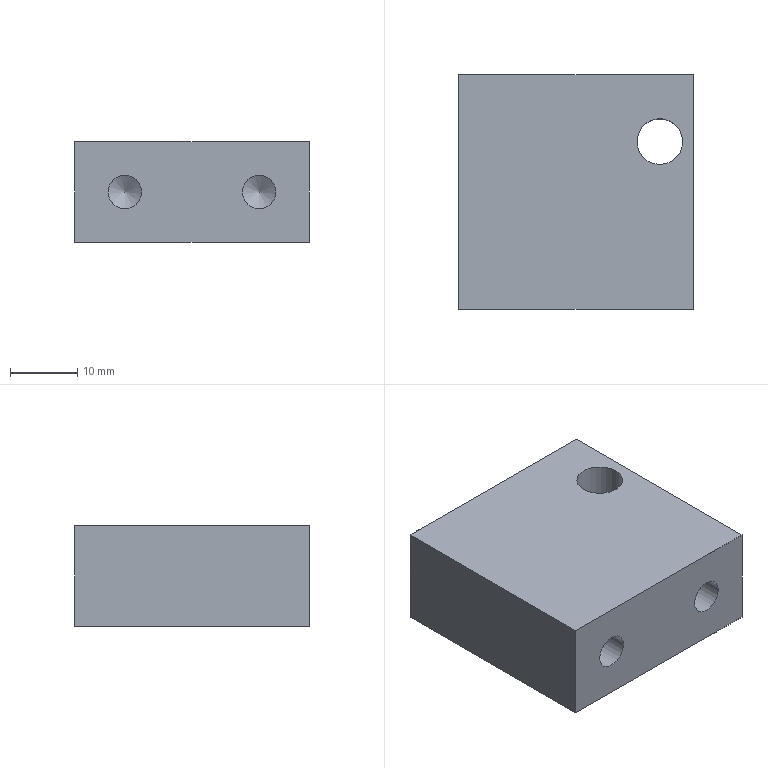Part | NX | features 5003_216_Bracket 2 | 1 solid | 11 faces | box 35 x 35 x 15 mm | volume 17222 mm3 | plane 6 | cylinder 3 | cone 2 | commonest cylinder face diameters 5 x2 6.8 x1
STEP:
#1=CARTESIAN_POINT('',(-185.615,28.9,-84.5));
#2=VERTEX_POINT('',#1);
#3=CARTESIAN_POINT('',(-185.615,-6.1,-84.5));
#4=VERTEX_POINT('',#3);
#5=CARTESIAN_POINT('',(-185.615,-6.1,-84.5));
#6=DIRECTION('',(0.,-1.,0.));
#7=VECTOR('',#6,1000.);
#8=LINE('',#5,#7);
#9=EDGE_CURVE('',#2,#4,#8,.T.);
#10=ORIENTED_EDGE('',*,*,#9,.T.);
#11=CARTESIAN_POINT('',(-185.615,-6.1,-69.5));
#12=VERTEX_POINT('',#11);
#13=CARTESIAN_POINT('',(-185.615,-6.1,-69.5));
#14=DIRECTION('',(0.,0.,-1.));
#15=VECTOR('',#14,1000.);
#16=LINE('',#13,#15);
#17=EDGE_CURVE('',#12,#4,#16,.T.);
#18=ORIENTED_EDGE('',*,*,#17,.F.);
#19=CARTESIAN_POINT('',(-185.615,28.9,-69.5));
#20=VERTEX_POINT('',#19);
#21=CARTESIAN_POINT('',(-185.615,-6.1,-69.5));
#22=DIRECTION('',(0.,-1.,0.));
#23=VECTOR('',#22,1000.);
#24=LINE('',#21,#23);
#25=EDGE_CURVE('',#20,#12,#24,.T.);
#26=ORIENTED_EDGE('',*,*,#25,.F.);
#27=CARTESIAN_POINT('',(-185.615,28.9,-69.5));
#28=DIRECTION('',(0.,0.,-1.));
#29=VECTOR('',#28,1000.);
#30=LINE('',#27,#29);
#31=EDGE_CURVE('',#20,#2,#30,.T.);
#32=ORIENTED_EDGE('',*,*,#31,.T.);
#33=EDGE_LOOP('',(#10,#18,#26,#32));
#34=FACE_BOUND('',#33,.T.);
#35=CARTESIAN_POINT('',(-185.615,-6.1,-69.5));
#36=DIRECTION('',(1.,0.,0.));
#37=DIRECTION('',(0.,0.,-1.));
#38=AXIS2_PLACEMENT_3D('',#35,#36,#37);
#39=PLANE('',#38);
#40=ADVANCED_FACE('',(#34),#39,.F.);
#41=CARTESIAN_POINT('',(-178.115,-6.1,-79.5));
#42=VERTEX_POINT('',#41);
#43=CARTESIAN_POINT('',(-178.115,-6.1,-77.));
#44=DIRECTION('',(0.,-1.,0.));
#45=DIRECTION('',(0.,0.,-1.));
#46=AXIS2_PLACEMENT_3D('',#43,#44,#45);
#47=CIRCLE('',#46,2.5);
#48=EDGE_CURVE('',#42,#42,#47,.T.);
#49=ORIENTED_EDGE('',*,*,#48,.F.);
#50=EDGE_LOOP('',(#49));
#51=FACE_BOUND('',#50,.T.);
#52=CARTESIAN_POINT('',(-158.115,-6.1,-79.5));
#53=VERTEX_POINT('',#52);
#54=CARTESIAN_POINT('',(-158.115,-6.1,-77.));
#55=DIRECTION('',(0.,-1.,0.));
#56=DIRECTION('',(0.,0.,-1.));
#57=AXIS2_PLACEMENT_3D('',#54,#55,#56);
#58=CIRCLE('',#57,2.5);
#59=EDGE_CURVE('',#53,#53,#58,.T.);
#60=ORIENTED_EDGE('',*,*,#59,.F.);
#61=EDGE_LOOP('',(#60));
#62=FACE_BOUND('',#61,.T.);
#63=CARTESIAN_POINT('',(-150.615,-6.1,-84.5));
#64=VERTEX_POINT('',#63);
#65=CARTESIAN_POINT('',(-150.615,-6.1,-84.5));
#66=DIRECTION('',(1.,0.,0.));
#67=VECTOR('',#66,1000.);
#68=LINE('',#65,#67);
#69=EDGE_CURVE('',#4,#64,#68,.T.);
#70=ORIENTED_EDGE('',*,*,#69,.T.);
#71=CARTESIAN_POINT('',(-150.615,-6.1,-69.5));
#72=VERTEX_POINT('',#71);
#73=CARTESIAN_POINT('',(-150.615,-6.1,-69.5));
#74=DIRECTION('',(0.,0.,-1.));
#75=VECTOR('',#74,1000.);
#76=LINE('',#73,#75);
#77=EDGE_CURVE('',#72,#64,#76,.T.);
#78=ORIENTED_EDGE('',*,*,#77,.F.);
#79=CARTESIAN_POINT('',(-150.615,-6.1,-69.5));
#80=DIRECTION('',(1.,0.,0.));
#81=VECTOR('',#80,1000.);
#82=LINE('',#79,#81);
#83=EDGE_CURVE('',#12,#72,#82,.T.);
#84=ORIENTED_EDGE('',*,*,#83,.F.);
#85=ORIENTED_EDGE('',*,*,#17,.T.);
#86=EDGE_LOOP('',(#70,#78,#84,#85));
#87=FACE_BOUND('',#86,.T.);
#88=CARTESIAN_POINT('',(-150.615,-6.1,-69.5));
#89=DIRECTION('',(0.,1.,0.));
#90=DIRECTION('',(-1.,0.,0.));
#91=AXIS2_PLACEMENT_3D('',#88,#89,#90);
#92=PLANE('',#91);
#93=ADVANCED_FACE('',(#51,#62,#87),#92,.F.);
#94=CARTESIAN_POINT('',(-150.615,28.9,-84.5));
#95=VERTEX_POINT('',#94);
#96=CARTESIAN_POINT('',(-150.615,-6.1,-84.5));
#97=DIRECTION('',(0.,1.,0.));
#98=VECTOR('',#97,1000.);
#99=LINE('',#96,#98);
#100=EDGE_CURVE('',#64,#95,#99,.T.);
#101=ORIENTED_EDGE('',*,*,#100,.T.);
#102=CARTESIAN_POINT('',(-150.615,28.9,-69.5));
#103=VERTEX_POINT('',#102);
#104=CARTESIAN_POINT('',(-150.615,28.9,-69.5));
#105=DIRECTION('',(0.,0.,-1.));
#106=VECTOR('',#105,1000.);
#107=LINE('',#104,#106);
#108=EDGE_CURVE('',#103,#95,#107,.T.);
#109=ORIENTED_EDGE('',*,*,#108,.F.);
#110=CARTESIAN_POINT('',(-150.615,-6.1,-69.5));
#111=DIRECTION('',(0.,1.,0.));
#112=VECTOR('',#111,1000.);
#113=LINE('',#110,#112);
#114=EDGE_CURVE('',#72,#103,#113,.T.);
#115=ORIENTED_EDGE('',*,*,#114,.F.);
#116=ORIENTED_EDGE('',*,*,#77,.T.);
#117=EDGE_LOOP('',(#101,#109,#115,#116));
#118=FACE_BOUND('',#117,.T.);
#119=CARTESIAN_POINT('',(-150.615,-6.1,-69.5));
#120=DIRECTION('',(-1.,0.,0.));
#121=DIRECTION('',(0.,0.,1.));
#122=AXIS2_PLACEMENT_3D('',#119,#120,#121);
#123=PLANE('',#122);
#124=ADVANCED_FACE('',(#118),#123,.F.);
#125=CARTESIAN_POINT('',(-150.615,28.9,-84.5));
#126=DIRECTION('',(-1.,0.,0.));
#127=VECTOR('',#126,1000.);
#128=LINE('',#125,#127);
#129=EDGE_CURVE('',#95,#2,#128,.T.);
#130=ORIENTED_EDGE('',*,*,#129,.T.);
#131=ORIENTED_EDGE('',*,*,#31,.F.);
#132=CARTESIAN_POINT('',(-150.615,28.9,-69.5));
#133=DIRECTION('',(-1.,0.,0.));
#134=VECTOR('',#133,1000.);
#135=LINE('',#132,#134);
#136=EDGE_CURVE('',#103,#20,#135,.T.);
#137=ORIENTED_EDGE('',*,*,#136,.F.);
#138=ORIENTED_EDGE('',*,*,#108,.T.);
#139=EDGE_LOOP('',(#130,#131,#137,#138));
#140=FACE_BOUND('',#139,.T.);
#141=CARTESIAN_POINT('',(-150.615,28.9,-69.5));
#142=DIRECTION('',(0.,-1.,0.));
#143=DIRECTION('',(1.,0.,0.));
#144=AXIS2_PLACEMENT_3D('',#141,#142,#143);
#145=PLANE('',#144);
#146=ADVANCED_FACE('',(#140),#145,.F.);
#147=CARTESIAN_POINT('',(-152.215,18.9,-69.5));
#148=VERTEX_POINT('',#147);
#149=CARTESIAN_POINT('',(-155.615,18.9,-69.5));
#150=DIRECTION('',(0.,0.,1.));
#151=DIRECTION('',(1.,0.,0.));
#152=AXIS2_PLACEMENT_3D('',#149,#150,#151);
#153=CIRCLE('',#152,3.4);
#154=EDGE_CURVE('',#148,#148,#153,.T.);
#155=ORIENTED_EDGE('',*,*,#154,.F.);
#156=EDGE_LOOP('',(#155));
#157=FACE_BOUND('',#156,.T.);
#158=ORIENTED_EDGE('',*,*,#25,.T.);
#159=ORIENTED_EDGE('',*,*,#83,.T.);
#160=ORIENTED_EDGE('',*,*,#114,.T.);
#161=ORIENTED_EDGE('',*,*,#136,.T.);
#162=EDGE_LOOP('',(#158,#159,#160,#161));
#163=FACE_BOUND('',#162,.T.);
#164=CARTESIAN_POINT('',(-168.115,11.4,-69.5));
#165=DIRECTION('',(0.,0.,1.));
#166=DIRECTION('',(1.,0.,0.));
#167=AXIS2_PLACEMENT_3D('',#164,#165,#166);
#168=PLANE('',#167);
#169=ADVANCED_FACE('',(#157,#163),#168,.T.);
#170=CARTESIAN_POINT('',(-152.215,18.9,-84.5));
#171=VERTEX_POINT('',#170);
#172=CARTESIAN_POINT('',(-155.615,18.9,-84.5));
#173=DIRECTION('',(0.,0.,1.));
#174=DIRECTION('',(1.,0.,0.));
#175=AXIS2_PLACEMENT_3D('',#172,#173,#174);
#176=CIRCLE('',#175,3.4);
#177=EDGE_CURVE('',#171,#171,#176,.T.);
#178=ORIENTED_EDGE('',*,*,#177,.T.);
#179=EDGE_LOOP('',(#178));
#180=FACE_BOUND('',#179,.T.);
#181=ORIENTED_EDGE('',*,*,#9,.F.);
#182=ORIENTED_EDGE('',*,*,#129,.F.);
#183=ORIENTED_EDGE('',*,*,#100,.F.);
#184=ORIENTED_EDGE('',*,*,#69,.F.);
#185=EDGE_LOOP('',(#181,#182,#183,#184));
#186=FACE_BOUND('',#185,.T.);
#187=CARTESIAN_POINT('',(-168.115,11.4,-84.5));
#188=DIRECTION('',(0.,0.,1.));
#189=DIRECTION('',(1.,0.,0.));
#190=AXIS2_PLACEMENT_3D('',#187,#188,#189);
#191=PLANE('',#190);
#192=ADVANCED_FACE('',(#180,#186),#191,.F.);
#193=CARTESIAN_POINT('',(-158.115,10.402,-77.));
#194=VERTEX_POINT('',#193);
#195=VERTEX_LOOP('',#194);
#196=FACE_BOUND('',#195,.T.);
#197=CARTESIAN_POINT('',(-158.115,8.9,-79.5));
#198=VERTEX_POINT('',#197);
#199=CARTESIAN_POINT('',(-158.115,8.9,-77.));
#200=DIRECTION('',(0.,-1.,0.));
#201=DIRECTION('',(0.,0.,-1.));
#202=AXIS2_PLACEMENT_3D('',#199,#200,#201);
#203=CIRCLE('',#202,2.5);
#204=EDGE_CURVE('',#198,#198,#203,.T.);
#205=ORIENTED_EDGE('',*,*,#204,.T.);
#206=EDGE_LOOP('',(#205));
#207=FACE_BOUND('',#206,.T.);
#208=CARTESIAN_POINT('',(-158.115,8.9,-77.));
#209=DIRECTION('',(0.,-1.,0.));
#210=DIRECTION('',(0.,0.,-1.));
#211=AXIS2_PLACEMENT_3D('',#208,#209,#210);
#212=CONICAL_SURFACE('',#211,2.5,1.03);
#213=ADVANCED_FACE('',(#196,#207),#212,.F.);
#214=ORIENTED_EDGE('',*,*,#204,.F.);
#215=EDGE_LOOP('',(#214));
#216=FACE_BOUND('',#215,.T.);
#217=ORIENTED_EDGE('',*,*,#59,.T.);
#218=EDGE_LOOP('',(#217));
#219=FACE_BOUND('',#218,.T.);
#220=CARTESIAN_POINT('',(-158.115,-6.1,-77.));
#221=DIRECTION('',(0.,-1.,0.));
#222=DIRECTION('',(0.,0.,-1.));
#223=AXIS2_PLACEMENT_3D('',#220,#221,#222);
#224=CYLINDRICAL_SURFACE('',#223,2.5);
#225=ADVANCED_FACE('',(#216,#219),#224,.F.);
#226=CARTESIAN_POINT('',(-178.115,10.402,-77.));
#227=VERTEX_POINT('',#226);
#228=VERTEX_LOOP('',#227);
#229=FACE_BOUND('',#228,.T.);
#230=CARTESIAN_POINT('',(-178.115,8.9,-79.5));
#231=VERTEX_POINT('',#230);
#232=CARTESIAN_POINT('',(-178.115,8.9,-77.));
#233=DIRECTION('',(0.,-1.,0.));
#234=DIRECTION('',(0.,0.,-1.));
#235=AXIS2_PLACEMENT_3D('',#232,#233,#234);
#236=CIRCLE('',#235,2.5);
#237=EDGE_CURVE('',#231,#231,#236,.T.);
#238=ORIENTED_EDGE('',*,*,#237,.T.);
#239=EDGE_LOOP('',(#238));
#240=FACE_BOUND('',#239,.T.);
#241=CARTESIAN_POINT('',(-178.115,8.9,-77.));
#242=DIRECTION('',(0.,-1.,0.));
#243=DIRECTION('',(0.,0.,-1.));
#244=AXIS2_PLACEMENT_3D('',#241,#242,#243);
#245=CONICAL_SURFACE('',#244,2.5,1.03);
#246=ADVANCED_FACE('',(#229,#240),#245,.F.);
#247=ORIENTED_EDGE('',*,*,#237,.F.);
#248=EDGE_LOOP('',(#247));
#249=FACE_BOUND('',#248,.T.);
#250=ORIENTED_EDGE('',*,*,#48,.T.);
#251=EDGE_LOOP('',(#250));
#252=FACE_BOUND('',#251,.T.);
#253=CARTESIAN_POINT('',(-178.115,-6.1,-77.));
#254=DIRECTION('',(0.,-1.,0.));
#255=DIRECTION('',(0.,0.,-1.));
#256=AXIS2_PLACEMENT_3D('',#253,#254,#255);
#257=CYLINDRICAL_SURFACE('',#256,2.5);
#258=ADVANCED_FACE('',(#249,#252),#257,.F.);
#259=ORIENTED_EDGE('',*,*,#177,.F.);
#260=EDGE_LOOP('',(#259));
#261=FACE_BOUND('',#260,.T.);
#262=ORIENTED_EDGE('',*,*,#154,.T.);
#263=EDGE_LOOP('',(#262));
#264=FACE_BOUND('',#263,.T.);
#265=CARTESIAN_POINT('',(-155.615,18.9,-69.5));
#266=DIRECTION('',(0.,0.,1.));
#267=DIRECTION('',(1.,0.,0.));
#268=AXIS2_PLACEMENT_3D('',#265,#266,#267);
#269=CYLINDRICAL_SURFACE('',#268,3.4);
#270=ADVANCED_FACE('',(#261,#264),#269,.F.);
#271=CLOSED_SHELL('',(#40,#93,#124,#146,#169,#192,#213,#225,#246,#258,#270));
#272=MANIFOLD_SOLID_BREP('',#271);
#273=(LENGTH_UNIT()NAMED_UNIT(*)SI_UNIT(.MILLI.,.METRE.));
#274=UNCERTAINTY_MEASURE_WITH_UNIT(LENGTH_MEASURE(0.00001),#273,'','');
#275=(NAMED_UNIT(*)PLANE_ANGLE_UNIT()SI_UNIT($,.RADIAN.));
#276=(NAMED_UNIT(*)SI_UNIT($,.STERADIAN.)SOLID_ANGLE_UNIT());
#277=(GEOMETRIC_REPRESENTATION_CONTEXT(3)GLOBAL_UNCERTAINTY_ASSIGNED_CONTEXT((#274))GLOBAL_UNIT_ASSIGNED_CONTEXT((#273,#275,#276))REPRESENTATION_CONTEXT('',''));
#278=ADVANCED_BREP_SHAPE_REPRESENTATION('',(#272),#277);